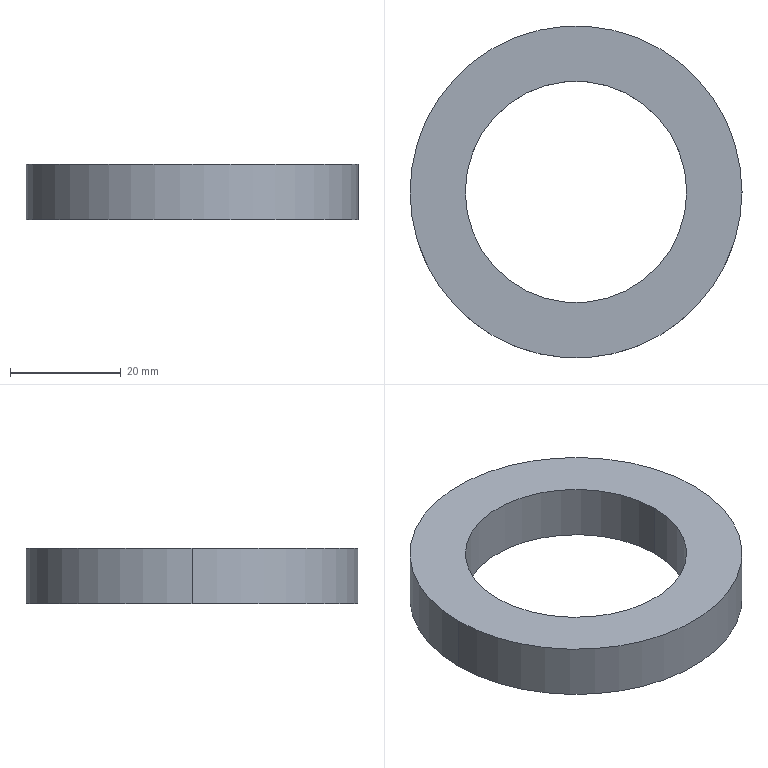Part | SolidWorks | features BaseBody 1 | 1 solid | 6 faces | box 60 x 60 x 10 mm | volume 15708 mm3 | cylinder 4 | plane 2 | commonest cylinder face diameters 40 x2 60 x2
STEP:
#1=CARTESIAN_POINT('',(20.,0.,10.));
#2=VERTEX_POINT('',#1);
#3=CARTESIAN_POINT('',(-20.,0.,10.));
#4=VERTEX_POINT('',#3);
#5=CARTESIAN_POINT('',(0.,0.,10.));
#6=DIRECTION('',(0.,0.,-1.));
#7=DIRECTION('',(-1.,0.,0.));
#8=AXIS2_PLACEMENT_3D('',#5,#6,#7);
#9=CIRCLE('',#8,20.);
#10=EDGE_CURVE('',#2,#4,#9,.T.);
#11=ORIENTED_EDGE('',*,*,#10,.F.);
#12=CARTESIAN_POINT('',(20.,0.,0.));
#13=VERTEX_POINT('',#12);
#14=CARTESIAN_POINT('',(20.,0.,10.));
#15=DIRECTION('',(0.,0.,-1.));
#16=VECTOR('',#15,1000.);
#17=LINE('',#14,#16);
#18=EDGE_CURVE('',#2,#13,#17,.T.);
#19=ORIENTED_EDGE('',*,*,#18,.T.);
#20=CARTESIAN_POINT('',(-20.,0.,0.));
#21=VERTEX_POINT('',#20);
#22=CARTESIAN_POINT('',(0.,0.,0.));
#23=DIRECTION('',(0.,0.,1.));
#24=DIRECTION('',(-1.,0.,0.));
#25=AXIS2_PLACEMENT_3D('',#22,#23,#24);
#26=CIRCLE('',#25,20.);
#27=EDGE_CURVE('',#21,#13,#26,.T.);
#28=ORIENTED_EDGE('',*,*,#27,.F.);
#29=CARTESIAN_POINT('',(-20.,0.,10.));
#30=DIRECTION('',(0.,0.,-1.));
#31=VECTOR('',#30,1000.);
#32=LINE('',#29,#31);
#33=EDGE_CURVE('',#4,#21,#32,.T.);
#34=ORIENTED_EDGE('',*,*,#33,.F.);
#35=EDGE_LOOP('',(#11,#19,#28,#34));
#36=FACE_OUTER_BOUND('',#35,.T.);
#37=CARTESIAN_POINT('',(0.,0.,10.));
#38=DIRECTION('',(0.,0.,-1.));
#39=DIRECTION('',(-1.,0.,0.));
#40=AXIS2_PLACEMENT_3D('',#37,#38,#39);
#41=CYLINDRICAL_SURFACE('',#40,20.);
#42=ADVANCED_FACE('',(#36),#41,.F.);
#43=CARTESIAN_POINT('',(30.,0.,10.));
#44=VERTEX_POINT('',#43);
#45=CARTESIAN_POINT('',(-30.,0.,10.));
#46=VERTEX_POINT('',#45);
#47=CARTESIAN_POINT('',(0.,0.,10.));
#48=DIRECTION('',(0.,0.,1.));
#49=DIRECTION('',(-1.,0.,0.));
#50=AXIS2_PLACEMENT_3D('',#47,#48,#49);
#51=CIRCLE('',#50,30.);
#52=EDGE_CURVE('',#44,#46,#51,.T.);
#53=ORIENTED_EDGE('',*,*,#52,.F.);
#54=CARTESIAN_POINT('',(30.,0.,0.));
#55=VERTEX_POINT('',#54);
#56=CARTESIAN_POINT('',(30.,0.,10.));
#57=DIRECTION('',(0.,0.,-1.));
#58=VECTOR('',#57,1000.);
#59=LINE('',#56,#58);
#60=EDGE_CURVE('',#44,#55,#59,.T.);
#61=ORIENTED_EDGE('',*,*,#60,.T.);
#62=CARTESIAN_POINT('',(-30.,0.,0.));
#63=VERTEX_POINT('',#62);
#64=CARTESIAN_POINT('',(0.,0.,0.));
#65=DIRECTION('',(0.,0.,1.));
#66=DIRECTION('',(-1.,0.,0.));
#67=AXIS2_PLACEMENT_3D('',#64,#65,#66);
#68=CIRCLE('',#67,30.);
#69=EDGE_CURVE('',#55,#63,#68,.T.);
#70=ORIENTED_EDGE('',*,*,#69,.T.);
#71=CARTESIAN_POINT('',(-30.,0.,10.));
#72=DIRECTION('',(0.,0.,-1.));
#73=VECTOR('',#72,1000.);
#74=LINE('',#71,#73);
#75=EDGE_CURVE('',#46,#63,#74,.T.);
#76=ORIENTED_EDGE('',*,*,#75,.F.);
#77=EDGE_LOOP('',(#53,#61,#70,#76));
#78=FACE_OUTER_BOUND('',#77,.T.);
#79=CARTESIAN_POINT('',(0.,0.,10.));
#80=DIRECTION('',(0.,0.,-1.));
#81=DIRECTION('',(-1.,0.,0.));
#82=AXIS2_PLACEMENT_3D('',#79,#80,#81);
#83=CYLINDRICAL_SURFACE('',#82,30.);
#84=ADVANCED_FACE('',(#78),#83,.T.);
#85=CARTESIAN_POINT('',(0.,0.,10.));
#86=DIRECTION('',(0.,0.,-1.));
#87=DIRECTION('',(-1.,0.,0.));
#88=AXIS2_PLACEMENT_3D('',#85,#86,#87);
#89=CIRCLE('',#88,20.);
#90=EDGE_CURVE('',#4,#2,#89,.T.);
#91=ORIENTED_EDGE('',*,*,#90,.T.);
#92=ORIENTED_EDGE('',*,*,#10,.T.);
#93=EDGE_LOOP('',(#91,#92));
#94=FACE_BOUND('',#93,.T.);
#95=CARTESIAN_POINT('',(0.,0.,10.));
#96=DIRECTION('',(0.,0.,1.));
#97=DIRECTION('',(-1.,0.,0.));
#98=AXIS2_PLACEMENT_3D('',#95,#96,#97);
#99=CIRCLE('',#98,30.);
#100=EDGE_CURVE('',#46,#44,#99,.T.);
#101=ORIENTED_EDGE('',*,*,#100,.T.);
#102=ORIENTED_EDGE('',*,*,#52,.T.);
#103=EDGE_LOOP('',(#101,#102));
#104=FACE_OUTER_BOUND('',#103,.T.);
#105=CARTESIAN_POINT('',(0.,0.,10.));
#106=DIRECTION('',(0.,0.,1.));
#107=DIRECTION('',(1.,0.,0.));
#108=AXIS2_PLACEMENT_3D('',#105,#106,#107);
#109=PLANE('',#108);
#110=ADVANCED_FACE('',(#94,#104),#109,.T.);
#111=ORIENTED_EDGE('',*,*,#18,.F.);
#112=ORIENTED_EDGE('',*,*,#90,.F.);
#113=ORIENTED_EDGE('',*,*,#33,.T.);
#114=CARTESIAN_POINT('',(0.,0.,0.));
#115=DIRECTION('',(0.,0.,1.));
#116=DIRECTION('',(-1.,0.,0.));
#117=AXIS2_PLACEMENT_3D('',#114,#115,#116);
#118=CIRCLE('',#117,20.);
#119=EDGE_CURVE('',#13,#21,#118,.T.);
#120=ORIENTED_EDGE('',*,*,#119,.F.);
#121=EDGE_LOOP('',(#111,#112,#113,#120));
#122=FACE_OUTER_BOUND('',#121,.T.);
#123=CARTESIAN_POINT('',(0.,0.,10.));
#124=DIRECTION('',(0.,0.,-1.));
#125=DIRECTION('',(-1.,0.,0.));
#126=AXIS2_PLACEMENT_3D('',#123,#124,#125);
#127=CYLINDRICAL_SURFACE('',#126,20.);
#128=ADVANCED_FACE('',(#122),#127,.F.);
#129=ORIENTED_EDGE('',*,*,#60,.F.);
#130=ORIENTED_EDGE('',*,*,#100,.F.);
#131=ORIENTED_EDGE('',*,*,#75,.T.);
#132=CARTESIAN_POINT('',(0.,0.,0.));
#133=DIRECTION('',(0.,0.,1.));
#134=DIRECTION('',(-1.,0.,0.));
#135=AXIS2_PLACEMENT_3D('',#132,#133,#134);
#136=CIRCLE('',#135,30.);
#137=EDGE_CURVE('',#63,#55,#136,.T.);
#138=ORIENTED_EDGE('',*,*,#137,.T.);
#139=EDGE_LOOP('',(#129,#130,#131,#138));
#140=FACE_OUTER_BOUND('',#139,.T.);
#141=CARTESIAN_POINT('',(0.,0.,10.));
#142=DIRECTION('',(0.,0.,-1.));
#143=DIRECTION('',(-1.,0.,0.));
#144=AXIS2_PLACEMENT_3D('',#141,#142,#143);
#145=CYLINDRICAL_SURFACE('',#144,30.);
#146=ADVANCED_FACE('',(#140),#145,.T.);
#147=ORIENTED_EDGE('',*,*,#27,.T.);
#148=ORIENTED_EDGE('',*,*,#119,.T.);
#149=EDGE_LOOP('',(#147,#148));
#150=FACE_BOUND('',#149,.T.);
#151=ORIENTED_EDGE('',*,*,#137,.F.);
#152=ORIENTED_EDGE('',*,*,#69,.F.);
#153=EDGE_LOOP('',(#151,#152));
#154=FACE_OUTER_BOUND('',#153,.T.);
#155=CARTESIAN_POINT('',(0.,0.,0.));
#156=DIRECTION('',(0.,0.,1.));
#157=DIRECTION('',(1.,0.,0.));
#158=AXIS2_PLACEMENT_3D('',#155,#156,#157);
#159=PLANE('',#158);
#160=ADVANCED_FACE('',(#150,#154),#159,.F.);
#161=CLOSED_SHELL('',(#42,#84,#110,#128,#146,#160));
#162=MANIFOLD_SOLID_BREP('',#161);
#163=CARTESIAN_POINT('',(0.,0.,0.));
#164=DIRECTION('',(0.,0.,1.));
#165=DIRECTION('',(1.,0.,0.));
#166=AXIS2_PLACEMENT_3D('',#163,#164,#165);
#167=(LENGTH_UNIT()NAMED_UNIT(*)SI_UNIT(.MILLI.,.METRE.));
#168=UNCERTAINTY_MEASURE_WITH_UNIT(LENGTH_MEASURE(0.00001),#167,'','');
#169=(NAMED_UNIT(*)PLANE_ANGLE_UNIT()SI_UNIT($,.RADIAN.));
#170=(NAMED_UNIT(*)SI_UNIT($,.STERADIAN.)SOLID_ANGLE_UNIT());
#171=(GEOMETRIC_REPRESENTATION_CONTEXT(3)GLOBAL_UNCERTAINTY_ASSIGNED_CONTEXT((#168))GLOBAL_UNIT_ASSIGNED_CONTEXT((#167,#169,#170))REPRESENTATION_CONTEXT('',''));
#172=ADVANCED_BREP_SHAPE_REPRESENTATION('',(#162,#166),#171);